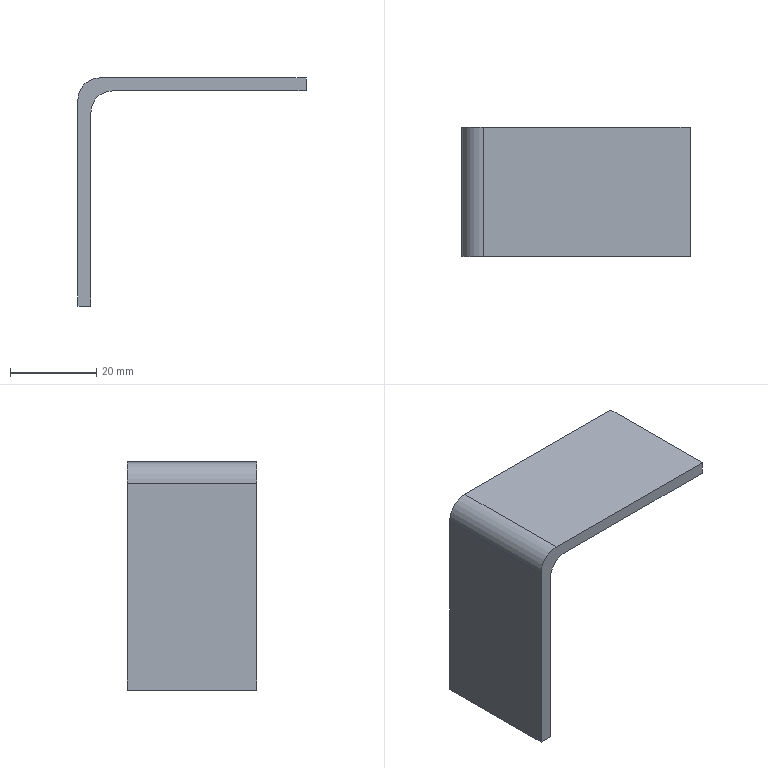Part | SolidWorks | features Extrusion 1 | 1 solid | 10 faces | box 53 x 30 x 53 mm | volume 9270 mm3 | plane 8 | cylinder 2 | commonest cylinder face diameters 10 x2
STEP:
#1=CARTESIAN_POINT('',(50.,0.,3.));
#2=VERTEX_POINT('',#1);
#3=CARTESIAN_POINT('',(50.,0.,0.));
#4=VERTEX_POINT('',#3);
#5=CARTESIAN_POINT('',(50.,0.,0.));
#6=DIRECTION('',(0.,0.,-1.));
#7=VECTOR('',#6,1000.);
#8=LINE('',#5,#7);
#9=EDGE_CURVE('',#2,#4,#8,.T.);
#10=ORIENTED_EDGE('',*,*,#9,.T.);
#11=CARTESIAN_POINT('',(50.,30.,0.));
#12=VERTEX_POINT('',#11);
#13=CARTESIAN_POINT('',(50.,30.,0.));
#14=DIRECTION('',(0.,-1.,0.));
#15=VECTOR('',#14,1000.);
#16=LINE('',#13,#15);
#17=EDGE_CURVE('',#12,#4,#16,.T.);
#18=ORIENTED_EDGE('',*,*,#17,.F.);
#19=CARTESIAN_POINT('',(50.,30.,3.));
#20=VERTEX_POINT('',#19);
#21=CARTESIAN_POINT('',(50.,30.,0.));
#22=DIRECTION('',(0.,0.,-1.));
#23=VECTOR('',#22,1000.);
#24=LINE('',#21,#23);
#25=EDGE_CURVE('',#20,#12,#24,.T.);
#26=ORIENTED_EDGE('',*,*,#25,.F.);
#27=CARTESIAN_POINT('',(50.,30.,3.));
#28=DIRECTION('',(0.,-1.,0.));
#29=VECTOR('',#28,1000.);
#30=LINE('',#27,#29);
#31=EDGE_CURVE('',#20,#2,#30,.T.);
#32=ORIENTED_EDGE('',*,*,#31,.T.);
#33=EDGE_LOOP('',(#10,#18,#26,#32));
#34=FACE_OUTER_BOUND('',#33,.T.);
#35=CARTESIAN_POINT('',(50.,30.,0.));
#36=DIRECTION('',(-1.,0.,0.));
#37=DIRECTION('',(0.,0.,1.));
#38=AXIS2_PLACEMENT_3D('',#35,#36,#37);
#39=PLANE('',#38);
#40=ADVANCED_FACE('',(#34),#39,.F.);
#41=CARTESIAN_POINT('',(5.,0.,0.));
#42=VERTEX_POINT('',#41);
#43=CARTESIAN_POINT('',(5.,0.,0.));
#44=DIRECTION('',(-1.,0.,0.));
#45=VECTOR('',#44,1000.);
#46=LINE('',#43,#45);
#47=EDGE_CURVE('',#4,#42,#46,.T.);
#48=ORIENTED_EDGE('',*,*,#47,.T.);
#49=CARTESIAN_POINT('',(5.,30.,0.));
#50=VERTEX_POINT('',#49);
#51=CARTESIAN_POINT('',(5.,30.,0.));
#52=DIRECTION('',(0.,-1.,0.));
#53=VECTOR('',#52,1000.);
#54=LINE('',#51,#53);
#55=EDGE_CURVE('',#50,#42,#54,.T.);
#56=ORIENTED_EDGE('',*,*,#55,.F.);
#57=CARTESIAN_POINT('',(5.,30.,0.));
#58=DIRECTION('',(-1.,0.,0.));
#59=VECTOR('',#58,1000.);
#60=LINE('',#57,#59);
#61=EDGE_CURVE('',#12,#50,#60,.T.);
#62=ORIENTED_EDGE('',*,*,#61,.F.);
#63=ORIENTED_EDGE('',*,*,#17,.T.);
#64=EDGE_LOOP('',(#48,#56,#62,#63));
#65=FACE_OUTER_BOUND('',#64,.T.);
#66=CARTESIAN_POINT('',(5.,30.,0.));
#67=DIRECTION('',(0.,0.,1.));
#68=DIRECTION('',(1.,0.,0.));
#69=AXIS2_PLACEMENT_3D('',#66,#67,#68);
#70=PLANE('',#69);
#71=ADVANCED_FACE('',(#65),#70,.F.);
#72=CARTESIAN_POINT('',(0.,0.,-5.));
#73=VERTEX_POINT('',#72);
#74=CARTESIAN_POINT('',(5.,0.,-5.));
#75=DIRECTION('',(0.,-1.,0.));
#76=DIRECTION('',(0.,0.,-1.));
#77=AXIS2_PLACEMENT_3D('',#74,#75,#76);
#78=CIRCLE('',#77,5.);
#79=EDGE_CURVE('',#42,#73,#78,.T.);
#80=ORIENTED_EDGE('',*,*,#79,.T.);
#81=CARTESIAN_POINT('',(0.,30.,-5.));
#82=VERTEX_POINT('',#81);
#83=CARTESIAN_POINT('',(0.,30.,-5.));
#84=DIRECTION('',(0.,-1.,0.));
#85=VECTOR('',#84,1000.);
#86=LINE('',#83,#85);
#87=EDGE_CURVE('',#82,#73,#86,.T.);
#88=ORIENTED_EDGE('',*,*,#87,.F.);
#89=CARTESIAN_POINT('',(5.,30.,-5.));
#90=DIRECTION('',(0.,-1.,0.));
#91=DIRECTION('',(0.,0.,-1.));
#92=AXIS2_PLACEMENT_3D('',#89,#90,#91);
#93=CIRCLE('',#92,5.);
#94=EDGE_CURVE('',#50,#82,#93,.T.);
#95=ORIENTED_EDGE('',*,*,#94,.F.);
#96=ORIENTED_EDGE('',*,*,#55,.T.);
#97=EDGE_LOOP('',(#80,#88,#95,#96));
#98=FACE_OUTER_BOUND('',#97,.T.);
#99=CARTESIAN_POINT('',(5.,30.,-5.));
#100=DIRECTION('',(0.,-1.,0.));
#101=DIRECTION('',(0.,0.,-1.));
#102=AXIS2_PLACEMENT_3D('',#99,#100,#101);
#103=CYLINDRICAL_SURFACE('',#102,5.);
#104=ADVANCED_FACE('',(#98),#103,.F.);
#105=CARTESIAN_POINT('',(0.,0.,-50.));
#106=VERTEX_POINT('',#105);
#107=CARTESIAN_POINT('',(0.,0.,-5.));
#108=DIRECTION('',(0.,0.,-1.));
#109=VECTOR('',#108,1000.);
#110=LINE('',#107,#109);
#111=EDGE_CURVE('',#73,#106,#110,.T.);
#112=ORIENTED_EDGE('',*,*,#111,.T.);
#113=CARTESIAN_POINT('',(0.,30.,-50.));
#114=VERTEX_POINT('',#113);
#115=CARTESIAN_POINT('',(0.,30.,-50.));
#116=DIRECTION('',(0.,-1.,0.));
#117=VECTOR('',#116,1000.);
#118=LINE('',#115,#117);
#119=EDGE_CURVE('',#114,#106,#118,.T.);
#120=ORIENTED_EDGE('',*,*,#119,.F.);
#121=CARTESIAN_POINT('',(0.,30.,-5.));
#122=DIRECTION('',(0.,0.,-1.));
#123=VECTOR('',#122,1000.);
#124=LINE('',#121,#123);
#125=EDGE_CURVE('',#82,#114,#124,.T.);
#126=ORIENTED_EDGE('',*,*,#125,.F.);
#127=ORIENTED_EDGE('',*,*,#87,.T.);
#128=EDGE_LOOP('',(#112,#120,#126,#127));
#129=FACE_OUTER_BOUND('',#128,.T.);
#130=CARTESIAN_POINT('',(0.,30.,-5.));
#131=DIRECTION('',(-1.,0.,0.));
#132=DIRECTION('',(0.,0.,1.));
#133=AXIS2_PLACEMENT_3D('',#130,#131,#132);
#134=PLANE('',#133);
#135=ADVANCED_FACE('',(#129),#134,.F.);
#136=CARTESIAN_POINT('',(-3.,0.,-50.));
#137=VERTEX_POINT('',#136);
#138=CARTESIAN_POINT('',(-3.,0.,-50.));
#139=DIRECTION('',(-1.,0.,0.));
#140=VECTOR('',#139,1000.);
#141=LINE('',#138,#140);
#142=EDGE_CURVE('',#106,#137,#141,.T.);
#143=ORIENTED_EDGE('',*,*,#142,.T.);
#144=CARTESIAN_POINT('',(-3.,30.,-50.));
#145=VERTEX_POINT('',#144);
#146=CARTESIAN_POINT('',(-3.,30.,-50.));
#147=DIRECTION('',(0.,-1.,0.));
#148=VECTOR('',#147,1000.);
#149=LINE('',#146,#148);
#150=EDGE_CURVE('',#145,#137,#149,.T.);
#151=ORIENTED_EDGE('',*,*,#150,.F.);
#152=CARTESIAN_POINT('',(-3.,30.,-50.));
#153=DIRECTION('',(-1.,0.,0.));
#154=VECTOR('',#153,1000.);
#155=LINE('',#152,#154);
#156=EDGE_CURVE('',#114,#145,#155,.T.);
#157=ORIENTED_EDGE('',*,*,#156,.F.);
#158=ORIENTED_EDGE('',*,*,#119,.T.);
#159=EDGE_LOOP('',(#143,#151,#157,#158));
#160=FACE_OUTER_BOUND('',#159,.T.);
#161=CARTESIAN_POINT('',(-3.,30.,-50.));
#162=DIRECTION('',(0.,0.,1.));
#163=DIRECTION('',(1.,0.,0.));
#164=AXIS2_PLACEMENT_3D('',#161,#162,#163);
#165=PLANE('',#164);
#166=ADVANCED_FACE('',(#160),#165,.F.);
#167=CARTESIAN_POINT('',(-3.,0.,-2.));
#168=VERTEX_POINT('',#167);
#169=CARTESIAN_POINT('',(-3.,0.,-2.));
#170=DIRECTION('',(0.,0.,1.));
#171=VECTOR('',#170,1000.);
#172=LINE('',#169,#171);
#173=EDGE_CURVE('',#137,#168,#172,.T.);
#174=ORIENTED_EDGE('',*,*,#173,.T.);
#175=CARTESIAN_POINT('',(-3.,30.,-2.));
#176=VERTEX_POINT('',#175);
#177=CARTESIAN_POINT('',(-3.,30.,-2.));
#178=DIRECTION('',(0.,-1.,0.));
#179=VECTOR('',#178,1000.);
#180=LINE('',#177,#179);
#181=EDGE_CURVE('',#176,#168,#180,.T.);
#182=ORIENTED_EDGE('',*,*,#181,.F.);
#183=CARTESIAN_POINT('',(-3.,30.,-2.));
#184=DIRECTION('',(0.,0.,1.));
#185=VECTOR('',#184,1000.);
#186=LINE('',#183,#185);
#187=EDGE_CURVE('',#145,#176,#186,.T.);
#188=ORIENTED_EDGE('',*,*,#187,.F.);
#189=ORIENTED_EDGE('',*,*,#150,.T.);
#190=EDGE_LOOP('',(#174,#182,#188,#189));
#191=FACE_OUTER_BOUND('',#190,.T.);
#192=CARTESIAN_POINT('',(-3.,30.,-2.));
#193=DIRECTION('',(1.,0.,0.));
#194=DIRECTION('',(0.,0.,-1.));
#195=AXIS2_PLACEMENT_3D('',#192,#193,#194);
#196=PLANE('',#195);
#197=ADVANCED_FACE('',(#191),#196,.F.);
#198=CARTESIAN_POINT('',(2.,0.,3.));
#199=VERTEX_POINT('',#198);
#200=CARTESIAN_POINT('',(2.,0.,-2.));
#201=DIRECTION('',(0.,1.,0.));
#202=DIRECTION('',(0.,0.,1.));
#203=AXIS2_PLACEMENT_3D('',#200,#201,#202);
#204=CIRCLE('',#203,5.);
#205=EDGE_CURVE('',#168,#199,#204,.T.);
#206=ORIENTED_EDGE('',*,*,#205,.T.);
#207=CARTESIAN_POINT('',(2.,30.,3.));
#208=VERTEX_POINT('',#207);
#209=CARTESIAN_POINT('',(2.,30.,3.));
#210=DIRECTION('',(0.,-1.,0.));
#211=VECTOR('',#210,1000.);
#212=LINE('',#209,#211);
#213=EDGE_CURVE('',#208,#199,#212,.T.);
#214=ORIENTED_EDGE('',*,*,#213,.F.);
#215=CARTESIAN_POINT('',(2.,30.,-2.));
#216=DIRECTION('',(0.,1.,0.));
#217=DIRECTION('',(0.,0.,1.));
#218=AXIS2_PLACEMENT_3D('',#215,#216,#217);
#219=CIRCLE('',#218,5.);
#220=EDGE_CURVE('',#176,#208,#219,.T.);
#221=ORIENTED_EDGE('',*,*,#220,.F.);
#222=ORIENTED_EDGE('',*,*,#181,.T.);
#223=EDGE_LOOP('',(#206,#214,#221,#222));
#224=FACE_OUTER_BOUND('',#223,.T.);
#225=CARTESIAN_POINT('',(2.,30.,-2.));
#226=DIRECTION('',(0.,-1.,0.));
#227=DIRECTION('',(0.,0.,-1.));
#228=AXIS2_PLACEMENT_3D('',#225,#226,#227);
#229=CYLINDRICAL_SURFACE('',#228,5.);
#230=ADVANCED_FACE('',(#224),#229,.T.);
#231=CARTESIAN_POINT('',(2.,0.,3.));
#232=DIRECTION('',(1.,0.,0.));
#233=VECTOR('',#232,1000.);
#234=LINE('',#231,#233);
#235=EDGE_CURVE('',#199,#2,#234,.T.);
#236=ORIENTED_EDGE('',*,*,#235,.T.);
#237=ORIENTED_EDGE('',*,*,#31,.F.);
#238=CARTESIAN_POINT('',(2.,30.,3.));
#239=DIRECTION('',(1.,0.,0.));
#240=VECTOR('',#239,1000.);
#241=LINE('',#238,#240);
#242=EDGE_CURVE('',#208,#20,#241,.T.);
#243=ORIENTED_EDGE('',*,*,#242,.F.);
#244=ORIENTED_EDGE('',*,*,#213,.T.);
#245=EDGE_LOOP('',(#236,#237,#243,#244));
#246=FACE_OUTER_BOUND('',#245,.T.);
#247=CARTESIAN_POINT('',(2.,30.,3.));
#248=DIRECTION('',(0.,0.,-1.));
#249=DIRECTION('',(-1.,0.,0.));
#250=AXIS2_PLACEMENT_3D('',#247,#248,#249);
#251=PLANE('',#250);
#252=ADVANCED_FACE('',(#246),#251,.F.);
#253=ORIENTED_EDGE('',*,*,#25,.T.);
#254=ORIENTED_EDGE('',*,*,#61,.T.);
#255=ORIENTED_EDGE('',*,*,#94,.T.);
#256=ORIENTED_EDGE('',*,*,#125,.T.);
#257=ORIENTED_EDGE('',*,*,#156,.T.);
#258=ORIENTED_EDGE('',*,*,#187,.T.);
#259=ORIENTED_EDGE('',*,*,#220,.T.);
#260=ORIENTED_EDGE('',*,*,#242,.T.);
#261=EDGE_LOOP('',(#253,#254,#255,#256,#257,#258,#259,#260));
#262=FACE_OUTER_BOUND('',#261,.T.);
#263=CARTESIAN_POINT('',(2.,30.,-2.));
#264=DIRECTION('',(0.,1.,0.));
#265=DIRECTION('',(0.,0.,1.));
#266=AXIS2_PLACEMENT_3D('',#263,#264,#265);
#267=PLANE('',#266);
#268=ADVANCED_FACE('',(#262),#267,.T.);
#269=ORIENTED_EDGE('',*,*,#9,.F.);
#270=ORIENTED_EDGE('',*,*,#235,.F.);
#271=ORIENTED_EDGE('',*,*,#205,.F.);
#272=ORIENTED_EDGE('',*,*,#173,.F.);
#273=ORIENTED_EDGE('',*,*,#142,.F.);
#274=ORIENTED_EDGE('',*,*,#111,.F.);
#275=ORIENTED_EDGE('',*,*,#79,.F.);
#276=ORIENTED_EDGE('',*,*,#47,.F.);
#277=EDGE_LOOP('',(#269,#270,#271,#272,#273,#274,#275,#276));
#278=FACE_OUTER_BOUND('',#277,.T.);
#279=CARTESIAN_POINT('',(2.,0.,-2.));
#280=DIRECTION('',(0.,1.,0.));
#281=DIRECTION('',(0.,0.,1.));
#282=AXIS2_PLACEMENT_3D('',#279,#280,#281);
#283=PLANE('',#282);
#284=ADVANCED_FACE('',(#278),#283,.F.);
#285=CLOSED_SHELL('',(#40,#71,#104,#135,#166,#197,#230,#252,#268,#284));
#286=MANIFOLD_SOLID_BREP('',#285);
#287=CARTESIAN_POINT('',(0.,0.,0.));
#288=DIRECTION('',(0.,0.,1.));
#289=DIRECTION('',(1.,0.,0.));
#290=AXIS2_PLACEMENT_3D('',#287,#288,#289);
#291=(LENGTH_UNIT()NAMED_UNIT(*)SI_UNIT(.MILLI.,.METRE.));
#292=UNCERTAINTY_MEASURE_WITH_UNIT(LENGTH_MEASURE(0.00001),#291,'','');
#293=(NAMED_UNIT(*)PLANE_ANGLE_UNIT()SI_UNIT($,.RADIAN.));
#294=(NAMED_UNIT(*)SI_UNIT($,.STERADIAN.)SOLID_ANGLE_UNIT());
#295=(GEOMETRIC_REPRESENTATION_CONTEXT(3)GLOBAL_UNCERTAINTY_ASSIGNED_CONTEXT((#292))GLOBAL_UNIT_ASSIGNED_CONTEXT((#291,#293,#294))REPRESENTATION_CONTEXT('',''));
#296=ADVANCED_BREP_SHAPE_REPRESENTATION('',(#286,#290),#295);